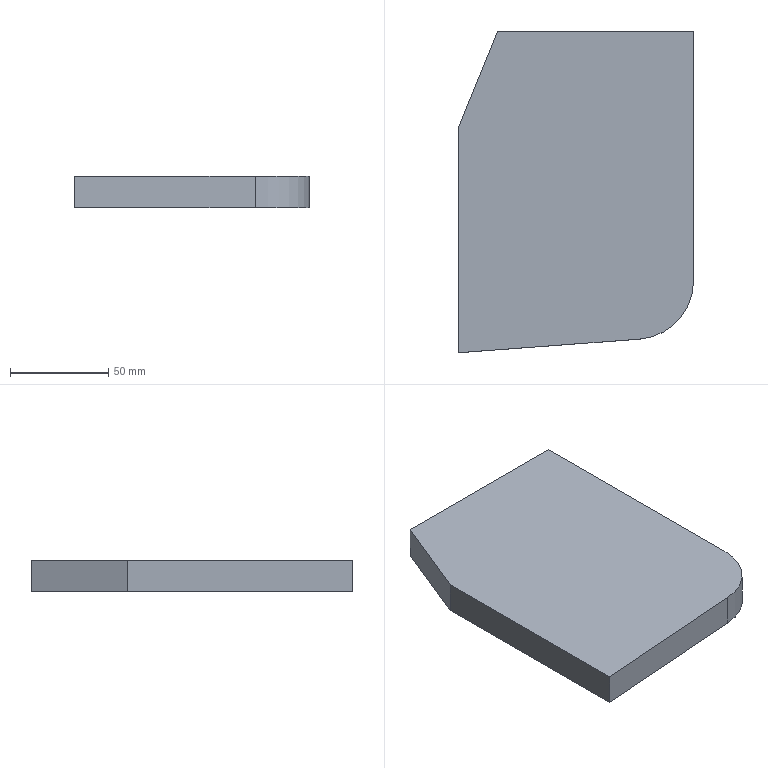Part | SolidWorks | features FlatPattern 1, SMBaseFlange 1, SheetMetal 1 | 1 solid | 8 faces | box 120 x 164 x 16 mm | volume 295810 mm3 | plane 7 | cylinder 1 | commonest cylinder face diameters 60 x1
STEP:
#1=CARTESIAN_POINT('',(0.,0.,0.));
#2=VERTEX_POINT('',#1);
#3=CARTESIAN_POINT('',(92.244,6.918,0.));
#4=VERTEX_POINT('',#3);
#5=CARTESIAN_POINT('',(92.244,6.918,0.));
#6=DIRECTION('',(0.9972,0.07479,0.));
#7=VECTOR('',#6,1000.);
#8=LINE('',#5,#7);
#9=EDGE_CURVE('',#2,#4,#8,.T.);
#10=ORIENTED_EDGE('',*,*,#9,.F.);
#11=CARTESIAN_POINT('',(0.,0.,-16.));
#12=VERTEX_POINT('',#11);
#13=CARTESIAN_POINT('',(0.,0.,-16.));
#14=DIRECTION('',(0.,0.,1.));
#15=VECTOR('',#14,1000.);
#16=LINE('',#13,#15);
#17=EDGE_CURVE('',#12,#2,#16,.T.);
#18=ORIENTED_EDGE('',*,*,#17,.F.);
#19=CARTESIAN_POINT('',(92.244,6.918,-16.));
#20=VERTEX_POINT('',#19);
#21=CARTESIAN_POINT('',(92.244,6.918,-16.));
#22=DIRECTION('',(0.9972,0.07479,0.));
#23=VECTOR('',#22,1000.);
#24=LINE('',#21,#23);
#25=EDGE_CURVE('',#12,#20,#24,.T.);
#26=ORIENTED_EDGE('',*,*,#25,.T.);
#27=CARTESIAN_POINT('',(92.244,6.918,-16.));
#28=DIRECTION('',(0.,0.,1.));
#29=VECTOR('',#28,1000.);
#30=LINE('',#27,#29);
#31=EDGE_CURVE('',#20,#4,#30,.T.);
#32=ORIENTED_EDGE('',*,*,#31,.T.);
#33=EDGE_LOOP('',(#10,#18,#26,#32));
#34=FACE_OUTER_BOUND('',#33,.T.);
#35=CARTESIAN_POINT('',(92.244,6.918,-16.));
#36=DIRECTION('',(0.07479,-0.9972,0.));
#37=DIRECTION('',(0.9972,0.07479,0.));
#38=AXIS2_PLACEMENT_3D('',#35,#36,#37);
#39=PLANE('',#38);
#40=ADVANCED_FACE('',(#34),#39,.T.);
#41=CARTESIAN_POINT('',(0.,115.,0.));
#42=VERTEX_POINT('',#41);
#43=CARTESIAN_POINT('',(0.,0.,0.));
#44=DIRECTION('',(0.,-1.,0.));
#45=VECTOR('',#44,1000.);
#46=LINE('',#43,#45);
#47=EDGE_CURVE('',#42,#2,#46,.T.);
#48=ORIENTED_EDGE('',*,*,#47,.F.);
#49=CARTESIAN_POINT('',(0.,115.,-16.));
#50=VERTEX_POINT('',#49);
#51=CARTESIAN_POINT('',(0.,115.,-16.));
#52=DIRECTION('',(0.,0.,1.));
#53=VECTOR('',#52,1000.);
#54=LINE('',#51,#53);
#55=EDGE_CURVE('',#50,#42,#54,.T.);
#56=ORIENTED_EDGE('',*,*,#55,.F.);
#57=CARTESIAN_POINT('',(0.,0.,-16.));
#58=DIRECTION('',(0.,-1.,0.));
#59=VECTOR('',#58,1000.);
#60=LINE('',#57,#59);
#61=EDGE_CURVE('',#50,#12,#60,.T.);
#62=ORIENTED_EDGE('',*,*,#61,.T.);
#63=ORIENTED_EDGE('',*,*,#17,.T.);
#64=EDGE_LOOP('',(#48,#56,#62,#63));
#65=FACE_OUTER_BOUND('',#64,.T.);
#66=CARTESIAN_POINT('',(0.,0.,-16.));
#67=DIRECTION('',(-1.,0.,0.));
#68=DIRECTION('',(0.,0.,1.));
#69=AXIS2_PLACEMENT_3D('',#66,#67,#68);
#70=PLANE('',#69);
#71=ADVANCED_FACE('',(#65),#70,.T.);
#72=CARTESIAN_POINT('',(20.,164.,0.));
#73=VERTEX_POINT('',#72);
#74=CARTESIAN_POINT('',(0.,115.,0.));
#75=DIRECTION('',(-0.3779,-0.9258,0.));
#76=VECTOR('',#75,1000.);
#77=LINE('',#74,#76);
#78=EDGE_CURVE('',#73,#42,#77,.T.);
#79=ORIENTED_EDGE('',*,*,#78,.F.);
#80=CARTESIAN_POINT('',(20.,164.,-16.));
#81=VERTEX_POINT('',#80);
#82=CARTESIAN_POINT('',(20.,164.,-16.));
#83=DIRECTION('',(0.,0.,1.));
#84=VECTOR('',#83,1000.);
#85=LINE('',#82,#84);
#86=EDGE_CURVE('',#81,#73,#85,.T.);
#87=ORIENTED_EDGE('',*,*,#86,.F.);
#88=CARTESIAN_POINT('',(0.,115.,-16.));
#89=DIRECTION('',(-0.3779,-0.9258,0.));
#90=VECTOR('',#89,1000.);
#91=LINE('',#88,#90);
#92=EDGE_CURVE('',#81,#50,#91,.T.);
#93=ORIENTED_EDGE('',*,*,#92,.T.);
#94=ORIENTED_EDGE('',*,*,#55,.T.);
#95=EDGE_LOOP('',(#79,#87,#93,#94));
#96=FACE_OUTER_BOUND('',#95,.T.);
#97=CARTESIAN_POINT('',(0.,115.,-16.));
#98=DIRECTION('',(-0.9258,0.3779,0.));
#99=DIRECTION('',(-0.3779,-0.9258,0.));
#100=AXIS2_PLACEMENT_3D('',#97,#98,#99);
#101=PLANE('',#100);
#102=ADVANCED_FACE('',(#96),#101,.T.);
#103=CARTESIAN_POINT('',(120.,164.,0.));
#104=VERTEX_POINT('',#103);
#105=CARTESIAN_POINT('',(20.,164.,0.));
#106=DIRECTION('',(-1.,0.,0.));
#107=VECTOR('',#106,1000.);
#108=LINE('',#105,#107);
#109=EDGE_CURVE('',#104,#73,#108,.T.);
#110=ORIENTED_EDGE('',*,*,#109,.F.);
#111=CARTESIAN_POINT('',(120.,164.,-16.));
#112=VERTEX_POINT('',#111);
#113=CARTESIAN_POINT('',(120.,164.,-16.));
#114=DIRECTION('',(0.,0.,1.));
#115=VECTOR('',#114,1000.);
#116=LINE('',#113,#115);
#117=EDGE_CURVE('',#112,#104,#116,.T.);
#118=ORIENTED_EDGE('',*,*,#117,.F.);
#119=CARTESIAN_POINT('',(20.,164.,-16.));
#120=DIRECTION('',(-1.,0.,0.));
#121=VECTOR('',#120,1000.);
#122=LINE('',#119,#121);
#123=EDGE_CURVE('',#112,#81,#122,.T.);
#124=ORIENTED_EDGE('',*,*,#123,.T.);
#125=ORIENTED_EDGE('',*,*,#86,.T.);
#126=EDGE_LOOP('',(#110,#118,#124,#125));
#127=FACE_OUTER_BOUND('',#126,.T.);
#128=CARTESIAN_POINT('',(20.,164.,-16.));
#129=DIRECTION('',(0.,1.,0.));
#130=DIRECTION('',(0.,0.,1.));
#131=AXIS2_PLACEMENT_3D('',#128,#129,#130);
#132=PLANE('',#131);
#133=ADVANCED_FACE('',(#127),#132,.T.);
#134=CARTESIAN_POINT('',(120.,36.834,0.));
#135=VERTEX_POINT('',#134);
#136=CARTESIAN_POINT('',(120.,164.,0.));
#137=DIRECTION('',(0.,1.,0.));
#138=VECTOR('',#137,1000.);
#139=LINE('',#136,#138);
#140=EDGE_CURVE('',#135,#104,#139,.T.);
#141=ORIENTED_EDGE('',*,*,#140,.F.);
#142=CARTESIAN_POINT('',(120.,36.834,-16.));
#143=VERTEX_POINT('',#142);
#144=CARTESIAN_POINT('',(120.,36.834,-16.));
#145=DIRECTION('',(0.,0.,1.));
#146=VECTOR('',#145,1000.);
#147=LINE('',#144,#146);
#148=EDGE_CURVE('',#143,#135,#147,.T.);
#149=ORIENTED_EDGE('',*,*,#148,.F.);
#150=CARTESIAN_POINT('',(120.,164.,-16.));
#151=DIRECTION('',(0.,1.,0.));
#152=VECTOR('',#151,1000.);
#153=LINE('',#150,#152);
#154=EDGE_CURVE('',#143,#112,#153,.T.);
#155=ORIENTED_EDGE('',*,*,#154,.T.);
#156=ORIENTED_EDGE('',*,*,#117,.T.);
#157=EDGE_LOOP('',(#141,#149,#155,#156));
#158=FACE_OUTER_BOUND('',#157,.T.);
#159=CARTESIAN_POINT('',(120.,164.,-16.));
#160=DIRECTION('',(1.,0.,0.));
#161=DIRECTION('',(0.,1.,0.));
#162=AXIS2_PLACEMENT_3D('',#159,#160,#161);
#163=PLANE('',#162);
#164=ADVANCED_FACE('',(#158),#163,.T.);
#165=CARTESIAN_POINT('',(90.,36.834,0.));
#166=DIRECTION('',(0.,0.,1.));
#167=DIRECTION('',(-1.,0.,0.));
#168=AXIS2_PLACEMENT_3D('',#165,#166,#167);
#169=CIRCLE('',#168,30.);
#170=EDGE_CURVE('',#4,#135,#169,.T.);
#171=ORIENTED_EDGE('',*,*,#170,.F.);
#172=ORIENTED_EDGE('',*,*,#31,.F.);
#173=CARTESIAN_POINT('',(90.,36.834,-16.));
#174=DIRECTION('',(0.,0.,1.));
#175=DIRECTION('',(-1.,0.,0.));
#176=AXIS2_PLACEMENT_3D('',#173,#174,#175);
#177=CIRCLE('',#176,30.);
#178=EDGE_CURVE('',#20,#143,#177,.T.);
#179=ORIENTED_EDGE('',*,*,#178,.T.);
#180=ORIENTED_EDGE('',*,*,#148,.T.);
#181=EDGE_LOOP('',(#171,#172,#179,#180));
#182=FACE_OUTER_BOUND('',#181,.T.);
#183=CARTESIAN_POINT('',(90.,36.834,-16.));
#184=DIRECTION('',(0.,0.,1.));
#185=DIRECTION('',(1.,0.,0.));
#186=AXIS2_PLACEMENT_3D('',#183,#184,#185);
#187=CYLINDRICAL_SURFACE('',#186,30.);
#188=ADVANCED_FACE('',(#182),#187,.T.);
#189=ORIENTED_EDGE('',*,*,#25,.F.);
#190=ORIENTED_EDGE('',*,*,#61,.F.);
#191=ORIENTED_EDGE('',*,*,#92,.F.);
#192=ORIENTED_EDGE('',*,*,#123,.F.);
#193=ORIENTED_EDGE('',*,*,#154,.F.);
#194=ORIENTED_EDGE('',*,*,#178,.F.);
#195=EDGE_LOOP('',(#189,#190,#191,#192,#193,#194));
#196=FACE_OUTER_BOUND('',#195,.T.);
#197=CARTESIAN_POINT('',(90.,36.834,-16.));
#198=DIRECTION('',(0.,0.,-1.));
#199=DIRECTION('',(-1.,0.,0.));
#200=AXIS2_PLACEMENT_3D('',#197,#198,#199);
#201=PLANE('',#200);
#202=ADVANCED_FACE('',(#196),#201,.T.);
#203=ORIENTED_EDGE('',*,*,#9,.T.);
#204=ORIENTED_EDGE('',*,*,#170,.T.);
#205=ORIENTED_EDGE('',*,*,#140,.T.);
#206=ORIENTED_EDGE('',*,*,#109,.T.);
#207=ORIENTED_EDGE('',*,*,#78,.T.);
#208=ORIENTED_EDGE('',*,*,#47,.T.);
#209=EDGE_LOOP('',(#203,#204,#205,#206,#207,#208));
#210=FACE_OUTER_BOUND('',#209,.T.);
#211=CARTESIAN_POINT('',(90.,36.834,0.));
#212=DIRECTION('',(0.,0.,-1.));
#213=DIRECTION('',(-1.,0.,0.));
#214=AXIS2_PLACEMENT_3D('',#211,#212,#213);
#215=PLANE('',#214);
#216=ADVANCED_FACE('',(#210),#215,.F.);
#217=CLOSED_SHELL('',(#40,#71,#102,#133,#164,#188,#202,#216));
#218=MANIFOLD_SOLID_BREP('',#217);
#219=CARTESIAN_POINT('',(0.,0.,0.));
#220=DIRECTION('',(0.,0.,1.));
#221=DIRECTION('',(1.,0.,0.));
#222=AXIS2_PLACEMENT_3D('',#219,#220,#221);
#223=(LENGTH_UNIT()NAMED_UNIT(*)SI_UNIT(.MILLI.,.METRE.));
#224=UNCERTAINTY_MEASURE_WITH_UNIT(LENGTH_MEASURE(0.00001),#223,'','');
#225=(NAMED_UNIT(*)PLANE_ANGLE_UNIT()SI_UNIT($,.RADIAN.));
#226=(NAMED_UNIT(*)SI_UNIT($,.STERADIAN.)SOLID_ANGLE_UNIT());
#227=(GEOMETRIC_REPRESENTATION_CONTEXT(3)GLOBAL_UNCERTAINTY_ASSIGNED_CONTEXT((#224))GLOBAL_UNIT_ASSIGNED_CONTEXT((#223,#225,#226))REPRESENTATION_CONTEXT('',''));
#228=ADVANCED_BREP_SHAPE_REPRESENTATION('',(#218,#222),#227);